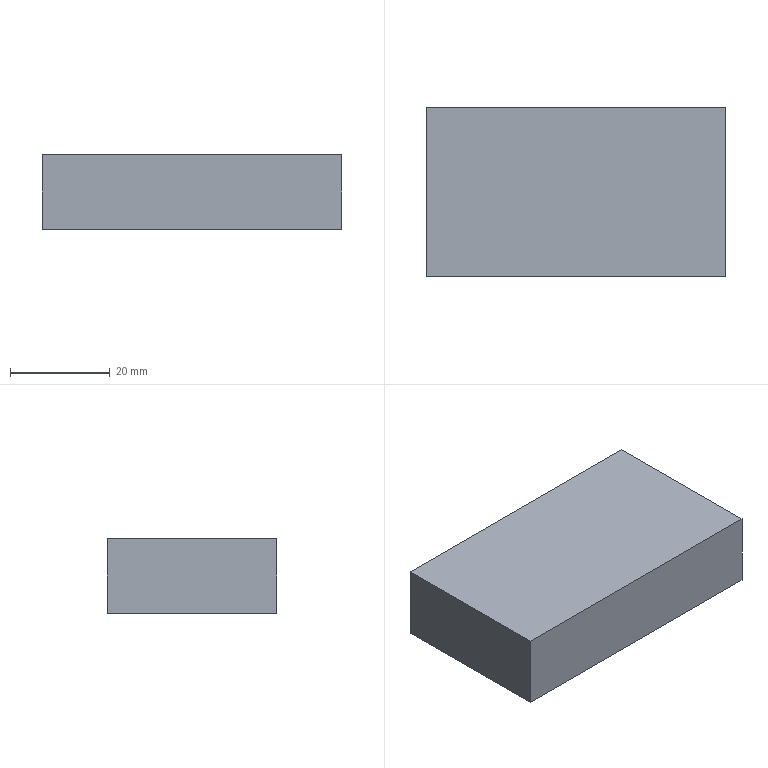Part | SolidWorks | features Extrusion 1 | 1 solid | 6 faces | box 60 x 34 x 15 mm | volume 30600 mm3 | plane 6
STEP:
#1=CARTESIAN_POINT('',(-30.,17.,0.));
#2=VERTEX_POINT('',#1);
#3=CARTESIAN_POINT('',(-30.,-17.,0.));
#4=VERTEX_POINT('',#3);
#5=CARTESIAN_POINT('',(-30.,-17.,0.));
#6=DIRECTION('',(0.,-1.,0.));
#7=VECTOR('',#6,1000.);
#8=LINE('',#5,#7);
#9=EDGE_CURVE('',#2,#4,#8,.T.);
#10=ORIENTED_EDGE('',*,*,#9,.T.);
#11=CARTESIAN_POINT('',(-30.,-17.,15.));
#12=VERTEX_POINT('',#11);
#13=CARTESIAN_POINT('',(-30.,-17.,15.));
#14=DIRECTION('',(0.,0.,-1.));
#15=VECTOR('',#14,1000.);
#16=LINE('',#13,#15);
#17=EDGE_CURVE('',#12,#4,#16,.T.);
#18=ORIENTED_EDGE('',*,*,#17,.F.);
#19=CARTESIAN_POINT('',(-30.,17.,15.));
#20=VERTEX_POINT('',#19);
#21=CARTESIAN_POINT('',(-30.,-17.,15.));
#22=DIRECTION('',(0.,-1.,0.));
#23=VECTOR('',#22,1000.);
#24=LINE('',#21,#23);
#25=EDGE_CURVE('',#20,#12,#24,.T.);
#26=ORIENTED_EDGE('',*,*,#25,.F.);
#27=CARTESIAN_POINT('',(-30.,17.,15.));
#28=DIRECTION('',(0.,0.,-1.));
#29=VECTOR('',#28,1000.);
#30=LINE('',#27,#29);
#31=EDGE_CURVE('',#20,#2,#30,.T.);
#32=ORIENTED_EDGE('',*,*,#31,.T.);
#33=EDGE_LOOP('',(#10,#18,#26,#32));
#34=FACE_OUTER_BOUND('',#33,.T.);
#35=CARTESIAN_POINT('',(-30.,-17.,15.));
#36=DIRECTION('',(1.,0.,0.));
#37=DIRECTION('',(0.,0.,-1.));
#38=AXIS2_PLACEMENT_3D('',#35,#36,#37);
#39=PLANE('',#38);
#40=ADVANCED_FACE('',(#34),#39,.F.);
#41=CARTESIAN_POINT('',(30.,-17.,0.));
#42=VERTEX_POINT('',#41);
#43=CARTESIAN_POINT('',(30.,-17.,0.));
#44=DIRECTION('',(1.,0.,0.));
#45=VECTOR('',#44,1000.);
#46=LINE('',#43,#45);
#47=EDGE_CURVE('',#4,#42,#46,.T.);
#48=ORIENTED_EDGE('',*,*,#47,.T.);
#49=CARTESIAN_POINT('',(30.,-17.,15.));
#50=VERTEX_POINT('',#49);
#51=CARTESIAN_POINT('',(30.,-17.,15.));
#52=DIRECTION('',(0.,0.,-1.));
#53=VECTOR('',#52,1000.);
#54=LINE('',#51,#53);
#55=EDGE_CURVE('',#50,#42,#54,.T.);
#56=ORIENTED_EDGE('',*,*,#55,.F.);
#57=CARTESIAN_POINT('',(30.,-17.,15.));
#58=DIRECTION('',(1.,0.,0.));
#59=VECTOR('',#58,1000.);
#60=LINE('',#57,#59);
#61=EDGE_CURVE('',#12,#50,#60,.T.);
#62=ORIENTED_EDGE('',*,*,#61,.F.);
#63=ORIENTED_EDGE('',*,*,#17,.T.);
#64=EDGE_LOOP('',(#48,#56,#62,#63));
#65=FACE_OUTER_BOUND('',#64,.T.);
#66=CARTESIAN_POINT('',(30.,-17.,15.));
#67=DIRECTION('',(0.,1.,0.));
#68=DIRECTION('',(-1.,0.,0.));
#69=AXIS2_PLACEMENT_3D('',#66,#67,#68);
#70=PLANE('',#69);
#71=ADVANCED_FACE('',(#65),#70,.F.);
#72=CARTESIAN_POINT('',(30.,17.,0.));
#73=VERTEX_POINT('',#72);
#74=CARTESIAN_POINT('',(30.,-17.,0.));
#75=DIRECTION('',(0.,1.,0.));
#76=VECTOR('',#75,1000.);
#77=LINE('',#74,#76);
#78=EDGE_CURVE('',#42,#73,#77,.T.);
#79=ORIENTED_EDGE('',*,*,#78,.T.);
#80=CARTESIAN_POINT('',(30.,17.,15.));
#81=VERTEX_POINT('',#80);
#82=CARTESIAN_POINT('',(30.,17.,15.));
#83=DIRECTION('',(0.,0.,-1.));
#84=VECTOR('',#83,1000.);
#85=LINE('',#82,#84);
#86=EDGE_CURVE('',#81,#73,#85,.T.);
#87=ORIENTED_EDGE('',*,*,#86,.F.);
#88=CARTESIAN_POINT('',(30.,-17.,15.));
#89=DIRECTION('',(0.,1.,0.));
#90=VECTOR('',#89,1000.);
#91=LINE('',#88,#90);
#92=EDGE_CURVE('',#50,#81,#91,.T.);
#93=ORIENTED_EDGE('',*,*,#92,.F.);
#94=ORIENTED_EDGE('',*,*,#55,.T.);
#95=EDGE_LOOP('',(#79,#87,#93,#94));
#96=FACE_OUTER_BOUND('',#95,.T.);
#97=CARTESIAN_POINT('',(30.,-17.,15.));
#98=DIRECTION('',(-1.,0.,0.));
#99=DIRECTION('',(0.,0.,1.));
#100=AXIS2_PLACEMENT_3D('',#97,#98,#99);
#101=PLANE('',#100);
#102=ADVANCED_FACE('',(#96),#101,.F.);
#103=CARTESIAN_POINT('',(30.,17.,0.));
#104=DIRECTION('',(-1.,0.,0.));
#105=VECTOR('',#104,1000.);
#106=LINE('',#103,#105);
#107=EDGE_CURVE('',#73,#2,#106,.T.);
#108=ORIENTED_EDGE('',*,*,#107,.T.);
#109=ORIENTED_EDGE('',*,*,#31,.F.);
#110=CARTESIAN_POINT('',(30.,17.,15.));
#111=DIRECTION('',(-1.,0.,0.));
#112=VECTOR('',#111,1000.);
#113=LINE('',#110,#112);
#114=EDGE_CURVE('',#81,#20,#113,.T.);
#115=ORIENTED_EDGE('',*,*,#114,.F.);
#116=ORIENTED_EDGE('',*,*,#86,.T.);
#117=EDGE_LOOP('',(#108,#109,#115,#116));
#118=FACE_OUTER_BOUND('',#117,.T.);
#119=CARTESIAN_POINT('',(30.,17.,15.));
#120=DIRECTION('',(0.,-1.,0.));
#121=DIRECTION('',(1.,0.,0.));
#122=AXIS2_PLACEMENT_3D('',#119,#120,#121);
#123=PLANE('',#122);
#124=ADVANCED_FACE('',(#118),#123,.F.);
#125=ORIENTED_EDGE('',*,*,#25,.T.);
#126=ORIENTED_EDGE('',*,*,#61,.T.);
#127=ORIENTED_EDGE('',*,*,#92,.T.);
#128=ORIENTED_EDGE('',*,*,#114,.T.);
#129=EDGE_LOOP('',(#125,#126,#127,#128));
#130=FACE_OUTER_BOUND('',#129,.T.);
#131=CARTESIAN_POINT('',(0.,0.,15.));
#132=DIRECTION('',(0.,0.,1.));
#133=DIRECTION('',(1.,0.,0.));
#134=AXIS2_PLACEMENT_3D('',#131,#132,#133);
#135=PLANE('',#134);
#136=ADVANCED_FACE('',(#130),#135,.T.);
#137=ORIENTED_EDGE('',*,*,#9,.F.);
#138=ORIENTED_EDGE('',*,*,#107,.F.);
#139=ORIENTED_EDGE('',*,*,#78,.F.);
#140=ORIENTED_EDGE('',*,*,#47,.F.);
#141=EDGE_LOOP('',(#137,#138,#139,#140));
#142=FACE_OUTER_BOUND('',#141,.T.);
#143=CARTESIAN_POINT('',(0.,0.,0.));
#144=DIRECTION('',(0.,0.,1.));
#145=DIRECTION('',(1.,0.,0.));
#146=AXIS2_PLACEMENT_3D('',#143,#144,#145);
#147=PLANE('',#146);
#148=ADVANCED_FACE('',(#142),#147,.F.);
#149=CLOSED_SHELL('',(#40,#71,#102,#124,#136,#148));
#150=MANIFOLD_SOLID_BREP('',#149);
#151=CARTESIAN_POINT('',(0.,0.,0.));
#152=DIRECTION('',(0.,0.,1.));
#153=DIRECTION('',(1.,0.,0.));
#154=AXIS2_PLACEMENT_3D('',#151,#152,#153);
#155=(LENGTH_UNIT()NAMED_UNIT(*)SI_UNIT(.MILLI.,.METRE.));
#156=UNCERTAINTY_MEASURE_WITH_UNIT(LENGTH_MEASURE(0.00001),#155,'','');
#157=(NAMED_UNIT(*)PLANE_ANGLE_UNIT()SI_UNIT($,.RADIAN.));
#158=(NAMED_UNIT(*)SI_UNIT($,.STERADIAN.)SOLID_ANGLE_UNIT());
#159=(GEOMETRIC_REPRESENTATION_CONTEXT(3)GLOBAL_UNCERTAINTY_ASSIGNED_CONTEXT((#156))GLOBAL_UNIT_ASSIGNED_CONTEXT((#155,#157,#158))REPRESENTATION_CONTEXT('',''));
#160=ADVANCED_BREP_SHAPE_REPRESENTATION('',(#150,#154),#159);